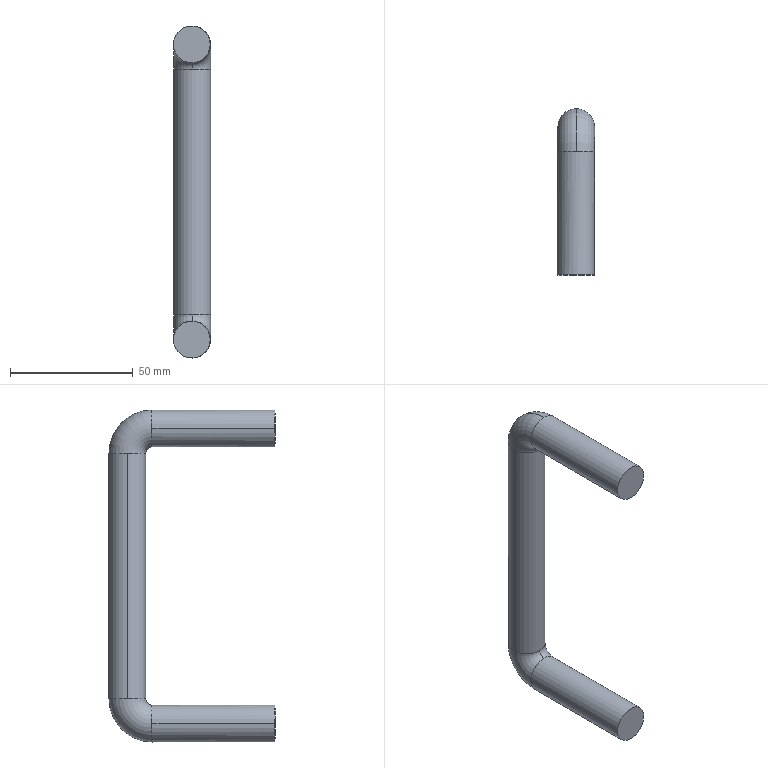Part | STEP file | Input 40 | 1 solid | 12 faces | box 15.178 x 67.522 x 135 mm | volume 40895 mm3 | cylinder 6 | torus 4 | plane 2 | commonest cylinder face diameters 15 x6
STEP:
#1=CARTESIAN_POINT('',(0.,0.,0.));
#2=DIRECTION('',(0.,0.,1.));
#3=DIRECTION('',(1.,0.,0.));
#4=AXIS2_PLACEMENT_3D('',#1,#2,#3);
#5=CARTESIAN_POINT('',(-3100.672,432.98,84.625));
#6=VERTEX_POINT('',#5);
#7=CARTESIAN_POINT('',(-3093.172,432.958,92.125));
#8=VERTEX_POINT('',#7);
#9=CARTESIAN_POINT('',(-3093.172,432.958,84.625));
#10=DIRECTION('',(0.002971,1.,0.));
#11=DIRECTION('',(-1.,0.002971,0.));
#12=AXIS2_PLACEMENT_3D('',#9,#10,#11);
#13=CIRCLE('',#12,7.5);
#14=CARTESIAN_POINT('',(-3093.172,432.958,74.625));
#15=DIRECTION('',(-1.,0.002971,0.));
#16=DIRECTION('',(0.,0.,1.));
#17=AXIS2_PLACEMENT_3D('',#14,#15,#16);
#18=TOROIDAL_SURFACE('',#17,10.,7.5);
#19=CARTESIAN_POINT('',(0.,1.571));
#20=CARTESIAN_POINT('',(0.,1.547));
#21=CARTESIAN_POINT('',(0.,1.499));
#22=CARTESIAN_POINT('',(0.,1.428));
#23=CARTESIAN_POINT('',(0.,1.357));
#24=CARTESIAN_POINT('',(0.,1.285));
#25=CARTESIAN_POINT('',(0.,1.214));
#26=CARTESIAN_POINT('',(0.,1.142));
#27=CARTESIAN_POINT('',(0.,1.071));
#28=CARTESIAN_POINT('',(0.,0.9996));
#29=CARTESIAN_POINT('',(0.,0.9282));
#30=CARTESIAN_POINT('',(0.,0.8568));
#31=CARTESIAN_POINT('',(0.,0.7854));
#32=CARTESIAN_POINT('',(0.,0.714));
#33=CARTESIAN_POINT('',(0.,0.6426));
#34=CARTESIAN_POINT('',(0.,0.5712));
#35=CARTESIAN_POINT('',(0.,0.4998));
#36=CARTESIAN_POINT('',(0.,0.4284));
#37=CARTESIAN_POINT('',(0.,0.357));
#38=CARTESIAN_POINT('',(0.,0.2856));
#39=CARTESIAN_POINT('',(0.,0.2142));
#40=CARTESIAN_POINT('',(0.,0.1428));
#41=CARTESIAN_POINT('',(0.,0.0714));
#42=CARTESIAN_POINT('',(0.,0.0238));
#43=CARTESIAN_POINT('',(0.,0.));
#44=B_SPLINE_CURVE_WITH_KNOTS('',3,(#19,#20,#21,#22,#23,#24,#25,#26,#27,#28,#29,#30,#31,#32,#33,#34,#35,#36,#37,#38,#39,#40,#41,#42,#43),.UNSPECIFIED.,.F.,.F.,(4,1,1,1,1,1,1,1,1,1,1,1,1,1,1,1,1,1,1,1,1,1,4),(0.,0.0714,0.1428,0.2142,0.2856,0.357,0.4284,0.4998,0.5712,0.6426,0.714,0.7854,0.8568,0.9282,0.9996,1.071,1.142,1.214,1.285,1.357,1.428,1.499,1.571),.QUASI_UNIFORM_KNOTS.);
#45=(GEOMETRIC_REPRESENTATION_CONTEXT(2)PARAMETRIC_REPRESENTATION_CONTEXT()REPRESENTATION_CONTEXT('',''));
#46=DEFINITIONAL_REPRESENTATION('',(#44),#45);
#47=PCURVE('',#18,#46);
#48=CARTESIAN_POINT('',(-3093.172,432.958,84.625));
#49=DIRECTION('',(-0.002971,-1.,0.));
#50=DIRECTION('',(1.,-0.002971,0.));
#51=AXIS2_PLACEMENT_3D('',#48,#49,#50);
#52=CYLINDRICAL_SURFACE('',#51,7.5);
#53=CARTESIAN_POINT('',(3.142,0.));
#54=DIRECTION('',(-1.,0.));
#55=VECTOR('',#54,1.);
#56=LINE('',#53,#55);
#57=(GEOMETRIC_REPRESENTATION_CONTEXT(2)PARAMETRIC_REPRESENTATION_CONTEXT()REPRESENTATION_CONTEXT('',''));
#58=DEFINITIONAL_REPRESENTATION('',(#56),#57);
#59=PCURVE('',#52,#58);
#60=SURFACE_CURVE('',#13,(#47,#59),.PCURVE_S1.);
#61=EDGE_CURVE('',#6,#8,#60,.T.);
#62=ORIENTED_EDGE('',*,*,#61,.T.);
#63=CARTESIAN_POINT('',(-3093.12,450.458,74.625));
#64=VERTEX_POINT('',#63);
#65=CARTESIAN_POINT('',(-3093.172,432.958,74.625));
#66=DIRECTION('',(-1.,0.002971,0.));
#67=DIRECTION('',(-0.002971,-1.,0.));
#68=AXIS2_PLACEMENT_3D('',#65,#66,#67);
#69=CIRCLE('',#68,17.5);
#70=CARTESIAN_POINT('',(-1.571,0.));
#71=DIRECTION('',(1.,0.));
#72=VECTOR('',#71,1.);
#73=LINE('',#70,#72);
#74=(GEOMETRIC_REPRESENTATION_CONTEXT(2)PARAMETRIC_REPRESENTATION_CONTEXT()REPRESENTATION_CONTEXT('',''));
#75=DEFINITIONAL_REPRESENTATION('',(#73),#74);
#76=PCURVE('',#18,#75);
#77=CARTESIAN_POINT('',(-3093.172,432.958,74.625));
#78=DIRECTION('',(-1.,0.002971,0.));
#79=DIRECTION('',(0.,0.,1.));
#80=AXIS2_PLACEMENT_3D('',#77,#78,#79);
#81=TOROIDAL_SURFACE('',#80,10.,7.5);
#82=CARTESIAN_POINT('',(-1.571,6.283));
#83=DIRECTION('',(1.,0.));
#84=VECTOR('',#83,1.);
#85=LINE('',#82,#84);
#86=(GEOMETRIC_REPRESENTATION_CONTEXT(2)PARAMETRIC_REPRESENTATION_CONTEXT()REPRESENTATION_CONTEXT('',''));
#87=DEFINITIONAL_REPRESENTATION('',(#85),#86);
#88=PCURVE('',#81,#87);
#89=SURFACE_CURVE('',#69,(#76,#88),.PCURVE_S1.);
#90=EDGE_CURVE('',#8,#64,#89,.T.);
#91=ORIENTED_EDGE('',*,*,#90,.T.);
#92=CARTESIAN_POINT('',(-3100.643,442.98,74.625));
#93=VERTEX_POINT('',#92);
#94=CARTESIAN_POINT('',(-3093.143,442.958,74.625));
#95=DIRECTION('',(0.,0.,-1.));
#96=DIRECTION('',(-1.,0.002971,0.));
#97=AXIS2_PLACEMENT_3D('',#94,#95,#96);
#98=CIRCLE('',#97,7.5);
#99=CARTESIAN_POINT('',(1.571,1.571));
#100=DIRECTION('',(0.,-1.));
#101=VECTOR('',#100,1.);
#102=LINE('',#99,#101);
#103=(GEOMETRIC_REPRESENTATION_CONTEXT(2)PARAMETRIC_REPRESENTATION_CONTEXT()REPRESENTATION_CONTEXT('',''));
#104=DEFINITIONAL_REPRESENTATION('',(#102),#103);
#105=PCURVE('',#18,#104);
#106=CARTESIAN_POINT('',(-3093.143,442.958,74.625));
#107=DIRECTION('',(0.,0.,-1.));
#108=DIRECTION('',(-1.,0.002971,0.));
#109=AXIS2_PLACEMENT_3D('',#106,#107,#108);
#110=CYLINDRICAL_SURFACE('',#109,7.5);
#111=CARTESIAN_POINT('',(0.,0.));
#112=DIRECTION('',(1.,0.));
#113=VECTOR('',#112,1.);
#114=LINE('',#111,#113);
#115=(GEOMETRIC_REPRESENTATION_CONTEXT(2)PARAMETRIC_REPRESENTATION_CONTEXT()REPRESENTATION_CONTEXT('',''));
#116=DEFINITIONAL_REPRESENTATION('',(#114),#115);
#117=PCURVE('',#110,#116);
#118=SURFACE_CURVE('',#98,(#105,#117),.PCURVE_S1.);
#119=EDGE_CURVE('',#93,#64,#118,.T.);
#120=ORIENTED_EDGE('',*,*,#119,.F.);
#121=CARTESIAN_POINT('',(-3093.165,435.458,74.625));
#122=VERTEX_POINT('',#121);
#123=CARTESIAN_POINT('',(-3093.143,442.958,74.625));
#124=DIRECTION('',(0.,0.,-1.));
#125=DIRECTION('',(-1.,0.002971,0.));
#126=AXIS2_PLACEMENT_3D('',#123,#124,#125);
#127=CIRCLE('',#126,7.5);
#128=CARTESIAN_POINT('',(1.571,7.854));
#129=DIRECTION('',(0.,-1.));
#130=VECTOR('',#129,1.);
#131=LINE('',#128,#130);
#132=(GEOMETRIC_REPRESENTATION_CONTEXT(2)PARAMETRIC_REPRESENTATION_CONTEXT()REPRESENTATION_CONTEXT('',''));
#133=DEFINITIONAL_REPRESENTATION('',(#131),#132);
#134=PCURVE('',#18,#133);
#135=CARTESIAN_POINT('',(-3093.143,442.958,74.625));
#136=DIRECTION('',(0.,0.,-1.));
#137=DIRECTION('',(-1.,0.002971,0.));
#138=AXIS2_PLACEMENT_3D('',#135,#136,#137);
#139=CYLINDRICAL_SURFACE('',#138,7.5);
#140=CARTESIAN_POINT('',(0.,0.));
#141=DIRECTION('',(1.,0.));
#142=VECTOR('',#141,1.);
#143=LINE('',#140,#142);
#144=(GEOMETRIC_REPRESENTATION_CONTEXT(2)PARAMETRIC_REPRESENTATION_CONTEXT()REPRESENTATION_CONTEXT('',''));
#145=DEFINITIONAL_REPRESENTATION('',(#143),#144);
#146=PCURVE('',#139,#145);
#147=SURFACE_CURVE('',#127,(#134,#146),.PCURVE_S1.);
#148=EDGE_CURVE('',#122,#93,#147,.T.);
#149=ORIENTED_EDGE('',*,*,#148,.F.);
#150=CARTESIAN_POINT('',(-3093.172,432.958,77.125));
#151=VERTEX_POINT('',#150);
#152=CARTESIAN_POINT('',(-3093.172,432.958,74.625));
#153=DIRECTION('',(-1.,0.002971,0.));
#154=DIRECTION('',(-0.002971,-1.,0.));
#155=AXIS2_PLACEMENT_3D('',#152,#153,#154);
#156=CIRCLE('',#155,2.5);
#157=CARTESIAN_POINT('',(-1.571,3.142));
#158=DIRECTION('',(1.,0.));
#159=VECTOR('',#158,1.);
#160=LINE('',#157,#159);
#161=(GEOMETRIC_REPRESENTATION_CONTEXT(2)PARAMETRIC_REPRESENTATION_CONTEXT()REPRESENTATION_CONTEXT('',''));
#162=DEFINITIONAL_REPRESENTATION('',(#160),#161);
#163=PCURVE('',#18,#162);
#164=CARTESIAN_POINT('',(-1.571,3.142));
#165=DIRECTION('',(1.,0.));
#166=VECTOR('',#165,1.);
#167=LINE('',#164,#166);
#168=(GEOMETRIC_REPRESENTATION_CONTEXT(2)PARAMETRIC_REPRESENTATION_CONTEXT()REPRESENTATION_CONTEXT('',''));
#169=DEFINITIONAL_REPRESENTATION('',(#167),#168);
#170=PCURVE('',#81,#169);
#171=SURFACE_CURVE('',#156,(#163,#170),.PCURVE_S1.);
#172=EDGE_CURVE('',#151,#122,#171,.T.);
#173=ORIENTED_EDGE('',*,*,#172,.F.);
#174=CARTESIAN_POINT('',(-3093.172,432.958,84.625));
#175=DIRECTION('',(0.002971,1.,0.));
#176=DIRECTION('',(-1.,0.002971,0.));
#177=AXIS2_PLACEMENT_3D('',#174,#175,#176);
#178=CIRCLE('',#177,7.5);
#179=CARTESIAN_POINT('',(0.,7.854));
#180=DIRECTION('',(0.,-1.));
#181=VECTOR('',#180,1.);
#182=LINE('',#179,#181);
#183=(GEOMETRIC_REPRESENTATION_CONTEXT(2)PARAMETRIC_REPRESENTATION_CONTEXT()REPRESENTATION_CONTEXT('',''));
#184=DEFINITIONAL_REPRESENTATION('',(#182),#183);
#185=PCURVE('',#18,#184);
#186=CARTESIAN_POINT('',(-3093.172,432.958,84.625));
#187=DIRECTION('',(-0.002971,-1.,0.));
#188=DIRECTION('',(1.,-0.002971,0.));
#189=AXIS2_PLACEMENT_3D('',#186,#187,#188);
#190=CYLINDRICAL_SURFACE('',#189,7.5);
#191=CARTESIAN_POINT('',(9.425,0.));
#192=DIRECTION('',(-1.,0.));
#193=VECTOR('',#192,1.);
#194=LINE('',#191,#193);
#195=(GEOMETRIC_REPRESENTATION_CONTEXT(2)PARAMETRIC_REPRESENTATION_CONTEXT()REPRESENTATION_CONTEXT('',''));
#196=DEFINITIONAL_REPRESENTATION('',(#194),#195);
#197=PCURVE('',#190,#196);
#198=SURFACE_CURVE('',#178,(#185,#197),.PCURVE_S1.);
#199=EDGE_CURVE('',#151,#6,#198,.T.);
#200=ORIENTED_EDGE('',*,*,#199,.T.);
#201=EDGE_LOOP('',(#62,#91,#120,#149,#173,#200));
#202=FACE_BOUND('',#201,.T.);
#203=ADVANCED_FACE('',(#202),#18,.T.);
#204=CARTESIAN_POINT('',(-3100.643,442.98,-25.375));
#205=VERTEX_POINT('',#204);
#206=CARTESIAN_POINT('',(-3093.12,450.458,-25.375));
#207=VERTEX_POINT('',#206);
#208=CARTESIAN_POINT('',(-3093.143,442.958,-25.375));
#209=DIRECTION('',(0.,0.,-1.));
#210=DIRECTION('',(-1.,0.002971,0.));
#211=AXIS2_PLACEMENT_3D('',#208,#209,#210);
#212=CIRCLE('',#211,7.5);
#213=CARTESIAN_POINT('',(-3093.172,432.958,-25.375));
#214=DIRECTION('',(-1.,0.002971,0.));
#215=DIRECTION('',(0.,0.,1.));
#216=AXIS2_PLACEMENT_3D('',#213,#214,#215);
#217=TOROIDAL_SURFACE('',#216,10.,7.5);
#218=CARTESIAN_POINT('',(1.571,1.571));
#219=DIRECTION('',(0.,-1.));
#220=VECTOR('',#219,1.);
#221=LINE('',#218,#220);
#222=(GEOMETRIC_REPRESENTATION_CONTEXT(2)PARAMETRIC_REPRESENTATION_CONTEXT()REPRESENTATION_CONTEXT('',''));
#223=DEFINITIONAL_REPRESENTATION('',(#221),#222);
#224=PCURVE('',#217,#223);
#225=CARTESIAN_POINT('',(0.,100.));
#226=DIRECTION('',(1.,0.));
#227=VECTOR('',#226,1.);
#228=LINE('',#225,#227);
#229=(GEOMETRIC_REPRESENTATION_CONTEXT(2)PARAMETRIC_REPRESENTATION_CONTEXT()REPRESENTATION_CONTEXT('',''));
#230=DEFINITIONAL_REPRESENTATION('',(#228),#229);
#231=PCURVE('',#110,#230);
#232=SURFACE_CURVE('',#212,(#224,#231),.PCURVE_S1.);
#233=EDGE_CURVE('',#205,#207,#232,.T.);
#234=ORIENTED_EDGE('',*,*,#233,.T.);
#235=CARTESIAN_POINT('',(-3093.172,432.958,-42.875));
#236=VERTEX_POINT('',#235);
#237=CARTESIAN_POINT('',(-3093.172,432.958,-25.375));
#238=DIRECTION('',(-1.,0.002971,0.));
#239=DIRECTION('',(-0.002971,-1.,0.));
#240=AXIS2_PLACEMENT_3D('',#237,#238,#239);
#241=CIRCLE('',#240,17.5);
#242=CARTESIAN_POINT('',(-1.571,0.));
#243=DIRECTION('',(1.,0.));
#244=VECTOR('',#243,1.);
#245=LINE('',#242,#244);
#246=(GEOMETRIC_REPRESENTATION_CONTEXT(2)PARAMETRIC_REPRESENTATION_CONTEXT()REPRESENTATION_CONTEXT('',''));
#247=DEFINITIONAL_REPRESENTATION('',(#245),#246);
#248=PCURVE('',#217,#247);
#249=CARTESIAN_POINT('',(-3093.172,432.958,-25.375));
#250=DIRECTION('',(-1.,0.002971,0.));
#251=DIRECTION('',(0.,0.,1.));
#252=AXIS2_PLACEMENT_3D('',#249,#250,#251);
#253=TOROIDAL_SURFACE('',#252,10.,7.5);
#254=CARTESIAN_POINT('',(-1.571,6.283));
#255=DIRECTION('',(1.,0.));
#256=VECTOR('',#255,1.);
#257=LINE('',#254,#256);
#258=(GEOMETRIC_REPRESENTATION_CONTEXT(2)PARAMETRIC_REPRESENTATION_CONTEXT()REPRESENTATION_CONTEXT('',''));
#259=DEFINITIONAL_REPRESENTATION('',(#257),#258);
#260=PCURVE('',#253,#259);
#261=SURFACE_CURVE('',#241,(#248,#260),.PCURVE_S1.);
#262=EDGE_CURVE('',#207,#236,#261,.T.);
#263=ORIENTED_EDGE('',*,*,#262,.T.);
#264=CARTESIAN_POINT('',(-3100.672,432.98,-35.375));
#265=VERTEX_POINT('',#264);
#266=CARTESIAN_POINT('',(-3093.172,432.958,-35.375));
#267=DIRECTION('',(-0.002971,-1.,0.));
#268=DIRECTION('',(-1.,0.002971,0.));
#269=AXIS2_PLACEMENT_3D('',#266,#267,#268);
#270=CIRCLE('',#269,7.5);
#271=CARTESIAN_POINT('',(3.142,1.571));
#272=DIRECTION('',(0.,-1.));
#273=VECTOR('',#272,1.);
#274=LINE('',#271,#273);
#275=(GEOMETRIC_REPRESENTATION_CONTEXT(2)PARAMETRIC_REPRESENTATION_CONTEXT()REPRESENTATION_CONTEXT('',''));
#276=DEFINITIONAL_REPRESENTATION('',(#274),#275);
#277=PCURVE('',#217,#276);
#278=CARTESIAN_POINT('',(-3093.172,432.958,-35.375));
#279=DIRECTION('',(-0.002971,-1.,0.));
#280=DIRECTION('',(1.,-0.002971,0.));
#281=AXIS2_PLACEMENT_3D('',#278,#279,#280);
#282=CYLINDRICAL_SURFACE('',#281,7.5);
#283=CARTESIAN_POINT('',(3.142,0.));
#284=DIRECTION('',(1.,0.));
#285=VECTOR('',#284,1.);
#286=LINE('',#283,#285);
#287=(GEOMETRIC_REPRESENTATION_CONTEXT(2)PARAMETRIC_REPRESENTATION_CONTEXT()REPRESENTATION_CONTEXT('',''));
#288=DEFINITIONAL_REPRESENTATION('',(#286),#287);
#289=PCURVE('',#282,#288);
#290=SURFACE_CURVE('',#270,(#277,#289),.PCURVE_S1.);
#291=EDGE_CURVE('',#265,#236,#290,.T.);
#292=ORIENTED_EDGE('',*,*,#291,.F.);
#293=CARTESIAN_POINT('',(-3093.172,432.958,-27.875));
#294=VERTEX_POINT('',#293);
#295=CARTESIAN_POINT('',(-3093.172,432.958,-35.375));
#296=DIRECTION('',(-0.002971,-1.,0.));
#297=DIRECTION('',(-1.,0.002971,0.));
#298=AXIS2_PLACEMENT_3D('',#295,#296,#297);
#299=CIRCLE('',#298,7.5);
#300=CARTESIAN_POINT('',(3.142,7.854));
#301=DIRECTION('',(0.,-1.));
#302=VECTOR('',#301,1.);
#303=LINE('',#300,#302);
#304=(GEOMETRIC_REPRESENTATION_CONTEXT(2)PARAMETRIC_REPRESENTATION_CONTEXT()REPRESENTATION_CONTEXT('',''));
#305=DEFINITIONAL_REPRESENTATION('',(#303),#304);
#306=PCURVE('',#217,#305);
#307=CARTESIAN_POINT('',(-3093.172,432.958,-35.375));
#308=DIRECTION('',(-0.002971,-1.,0.));
#309=DIRECTION('',(1.,-0.002971,0.));
#310=AXIS2_PLACEMENT_3D('',#307,#308,#309);
#311=CYLINDRICAL_SURFACE('',#310,7.5);
#312=CARTESIAN_POINT('',(-3.142,0.));
#313=DIRECTION('',(1.,0.));
#314=VECTOR('',#313,1.);
#315=LINE('',#312,#314);
#316=(GEOMETRIC_REPRESENTATION_CONTEXT(2)PARAMETRIC_REPRESENTATION_CONTEXT()REPRESENTATION_CONTEXT('',''));
#317=DEFINITIONAL_REPRESENTATION('',(#315),#316);
#318=PCURVE('',#311,#317);
#319=SURFACE_CURVE('',#299,(#306,#318),.PCURVE_S1.);
#320=EDGE_CURVE('',#294,#265,#319,.T.);
#321=ORIENTED_EDGE('',*,*,#320,.F.);
#322=CARTESIAN_POINT('',(-3093.165,435.458,-25.375));
#323=VERTEX_POINT('',#322);
#324=CARTESIAN_POINT('',(-3093.172,432.958,-25.375));
#325=DIRECTION('',(-1.,0.002971,0.));
#326=DIRECTION('',(-0.002971,-1.,0.));
#327=AXIS2_PLACEMENT_3D('',#324,#325,#326);
#328=CIRCLE('',#327,2.5);
#329=CARTESIAN_POINT('',(-1.571,3.142));
#330=DIRECTION('',(1.,0.));
#331=VECTOR('',#330,1.);
#332=LINE('',#329,#331);
#333=(GEOMETRIC_REPRESENTATION_CONTEXT(2)PARAMETRIC_REPRESENTATION_CONTEXT()REPRESENTATION_CONTEXT('',''));
#334=DEFINITIONAL_REPRESENTATION('',(#332),#333);
#335=PCURVE('',#217,#334);
#336=CARTESIAN_POINT('',(-1.571,3.142));
#337=DIRECTION('',(1.,0.));
#338=VECTOR('',#337,1.);
#339=LINE('',#336,#338);
#340=(GEOMETRIC_REPRESENTATION_CONTEXT(2)PARAMETRIC_REPRESENTATION_CONTEXT()REPRESENTATION_CONTEXT('',''));
#341=DEFINITIONAL_REPRESENTATION('',(#339),#340);
#342=PCURVE('',#253,#341);
#343=SURFACE_CURVE('',#328,(#335,#342),.PCURVE_S1.);
#344=EDGE_CURVE('',#323,#294,#343,.T.);
#345=ORIENTED_EDGE('',*,*,#344,.F.);
#346=CARTESIAN_POINT('',(-3093.143,442.958,-25.375));
#347=DIRECTION('',(0.,0.,-1.));
#348=DIRECTION('',(-1.,0.002971,0.));
#349=AXIS2_PLACEMENT_3D('',#346,#347,#348);
#350=CIRCLE('',#349,7.5);
#351=CARTESIAN_POINT('',(1.571,7.854));
#352=DIRECTION('',(0.,-1.));
#353=VECTOR('',#352,1.);
#354=LINE('',#351,#353);
#355=(GEOMETRIC_REPRESENTATION_CONTEXT(2)PARAMETRIC_REPRESENTATION_CONTEXT()REPRESENTATION_CONTEXT('',''));
#356=DEFINITIONAL_REPRESENTATION('',(#354),#355);
#357=PCURVE('',#217,#356);
#358=CARTESIAN_POINT('',(0.,100.));
#359=DIRECTION('',(1.,0.));
#360=VECTOR('',#359,1.);
#361=LINE('',#358,#360);
#362=(GEOMETRIC_REPRESENTATION_CONTEXT(2)PARAMETRIC_REPRESENTATION_CONTEXT()REPRESENTATION_CONTEXT('',''));
#363=DEFINITIONAL_REPRESENTATION('',(#361),#362);
#364=PCURVE('',#139,#363);
#365=SURFACE_CURVE('',#350,(#357,#364),.PCURVE_S1.);
#366=EDGE_CURVE('',#323,#205,#365,.T.);
#367=ORIENTED_EDGE('',*,*,#366,.T.);
#368=EDGE_LOOP('',(#234,#263,#292,#321,#345,#367));
#369=FACE_BOUND('',#368,.T.);
#370=ADVANCED_FACE('',(#369),#217,.T.);
#371=ORIENTED_EDGE('',*,*,#61,.F.);
#372=CARTESIAN_POINT('',(-3100.821,382.98,84.625));
#373=VERTEX_POINT('',#372);
#374=CARTESIAN_POINT('',(-3100.672,432.98,84.625));
#375=DIRECTION('',(-0.002971,-1.,0.));
#376=VECTOR('',#375,1.);
#377=LINE('',#374,#376);
#378=CARTESIAN_POINT('',(3.142,0.));
#379=DIRECTION('',(0.,1.));
#380=VECTOR('',#379,1.);
#381=LINE('',#378,#380);
#382=(GEOMETRIC_REPRESENTATION_CONTEXT(2)PARAMETRIC_REPRESENTATION_CONTEXT()REPRESENTATION_CONTEXT('',''));
#383=DEFINITIONAL_REPRESENTATION('',(#381),#382);
#384=PCURVE('',#52,#383);
#385=CARTESIAN_POINT('',(3.142,0.));
#386=DIRECTION('',(0.,1.));
#387=VECTOR('',#386,1.);
#388=LINE('',#385,#387);
#389=(GEOMETRIC_REPRESENTATION_CONTEXT(2)PARAMETRIC_REPRESENTATION_CONTEXT()REPRESENTATION_CONTEXT('',''));
#390=DEFINITIONAL_REPRESENTATION('',(#388),#389);
#391=PCURVE('',#190,#390);
#392=SURFACE_CURVE('',#377,(#384,#391),.PCURVE_S1.);
#393=EDGE_CURVE('',#6,#373,#392,.T.);
#394=ORIENTED_EDGE('',*,*,#393,.T.);
#395=CARTESIAN_POINT('',(-3085.821,382.936,84.625));
#396=VERTEX_POINT('',#395);
#397=CARTESIAN_POINT('',(-3093.321,382.958,84.625));
#398=DIRECTION('',(0.002971,1.,0.));
#399=DIRECTION('',(-1.,0.002971,0.));
#400=AXIS2_PLACEMENT_3D('',#397,#398,#399);
#401=CIRCLE('',#400,7.5);
#402=CARTESIAN_POINT('',(3.142,50.));
#403=DIRECTION('',(-1.,0.));
#404=VECTOR('',#403,1.);
#405=LINE('',#402,#404);
#406=(GEOMETRIC_REPRESENTATION_CONTEXT(2)PARAMETRIC_REPRESENTATION_CONTEXT()REPRESENTATION_CONTEXT('',''));
#407=DEFINITIONAL_REPRESENTATION('',(#405),#406);
#408=PCURVE('',#52,#407);
#409=CARTESIAN_POINT('',(-3093.321,382.958,84.625));
#410=DIRECTION('',(0.002971,1.,0.));
#411=DIRECTION('',(-1.,0.002971,0.));
#412=AXIS2_PLACEMENT_3D('',#409,#410,#411);
#413=PLANE('',#412);
#414=CARTESIAN_POINT('',(0.,0.));
#415=DIRECTION('',(1.,0.));
#416=AXIS2_PLACEMENT_2D('',#414,#415);
#417=CIRCLE('',#416,7.5);
#418=(GEOMETRIC_REPRESENTATION_CONTEXT(2)PARAMETRIC_REPRESENTATION_CONTEXT()REPRESENTATION_CONTEXT('',''));
#419=DEFINITIONAL_REPRESENTATION('',(#417),#418);
#420=PCURVE('',#413,#419);
#421=SURFACE_CURVE('',#401,(#408,#420),.PCURVE_S1.);
#422=EDGE_CURVE('',#373,#396,#421,.T.);
#423=ORIENTED_EDGE('',*,*,#422,.T.);
#424=CARTESIAN_POINT('',(-3085.672,432.936,84.625));
#425=VERTEX_POINT('',#424);
#426=CARTESIAN_POINT('',(-3085.672,432.936,84.625));
#427=DIRECTION('',(-0.002971,-1.,0.));
#428=VECTOR('',#427,1.);
#429=LINE('',#426,#428);
#430=CARTESIAN_POINT('',(0.,0.));
#431=DIRECTION('',(0.,1.));
#432=VECTOR('',#431,1.);
#433=LINE('',#430,#432);
#434=(GEOMETRIC_REPRESENTATION_CONTEXT(2)PARAMETRIC_REPRESENTATION_CONTEXT()REPRESENTATION_CONTEXT('',''));
#435=DEFINITIONAL_REPRESENTATION('',(#433),#434);
#436=PCURVE('',#52,#435);
#437=CARTESIAN_POINT('',(6.283,0.));
#438=DIRECTION('',(0.,1.));
#439=VECTOR('',#438,1.);
#440=LINE('',#437,#439);
#441=(GEOMETRIC_REPRESENTATION_CONTEXT(2)PARAMETRIC_REPRESENTATION_CONTEXT()REPRESENTATION_CONTEXT('',''));
#442=DEFINITIONAL_REPRESENTATION('',(#440),#441);
#443=PCURVE('',#190,#442);
#444=SURFACE_CURVE('',#429,(#436,#443),.PCURVE_S1.);
#445=EDGE_CURVE('',#425,#396,#444,.T.);
#446=ORIENTED_EDGE('',*,*,#445,.F.);
#447=CARTESIAN_POINT('',(-3093.172,432.958,84.625));
#448=DIRECTION('',(0.002971,1.,0.));
#449=DIRECTION('',(-1.,0.002971,0.));
#450=AXIS2_PLACEMENT_3D('',#447,#448,#449);
#451=CIRCLE('',#450,7.5);
#452=CARTESIAN_POINT('',(3.142,0.));
#453=DIRECTION('',(-1.,0.));
#454=VECTOR('',#453,1.);
#455=LINE('',#452,#454);
#456=(GEOMETRIC_REPRESENTATION_CONTEXT(2)PARAMETRIC_REPRESENTATION_CONTEXT()REPRESENTATION_CONTEXT('',''));
#457=DEFINITIONAL_REPRESENTATION('',(#455),#456);
#458=PCURVE('',#52,#457);
#459=CARTESIAN_POINT('',(0.,7.854));
#460=DIRECTION('',(0.,-1.));
#461=VECTOR('',#460,1.);
#462=LINE('',#459,#461);
#463=(GEOMETRIC_REPRESENTATION_CONTEXT(2)PARAMETRIC_REPRESENTATION_CONTEXT()REPRESENTATION_CONTEXT('',''));
#464=DEFINITIONAL_REPRESENTATION('',(#462),#463);
#465=PCURVE('',#81,#464);
#466=SURFACE_CURVE('',#451,(#458,#465),.PCURVE_S1.);
#467=EDGE_CURVE('',#8,#425,#466,.T.);
#468=ORIENTED_EDGE('',*,*,#467,.F.);
#469=EDGE_LOOP('',(#371,#394,#423,#446,#468));
#470=FACE_BOUND('',#469,.T.);
#471=ADVANCED_FACE('',(#470),#52,.T.);
#472=ORIENTED_EDGE('',*,*,#119,.T.);
#473=CARTESIAN_POINT('',(-3085.643,442.935,74.625));
#474=VERTEX_POINT('',#473);
#475=CARTESIAN_POINT('',(-3093.143,442.958,74.625));
#476=DIRECTION('',(0.,0.,-1.));
#477=DIRECTION('',(-1.,0.002971,0.));
#478=AXIS2_PLACEMENT_3D('',#475,#476,#477);
#479=CIRCLE('',#478,7.5);
#480=CARTESIAN_POINT('',(0.,0.));
#481=DIRECTION('',(1.,0.));
#482=VECTOR('',#481,1.);
#483=LINE('',#480,#482);
#484=(GEOMETRIC_REPRESENTATION_CONTEXT(2)PARAMETRIC_REPRESENTATION_CONTEXT()REPRESENTATION_CONTEXT('',''));
#485=DEFINITIONAL_REPRESENTATION('',(#483),#484);
#486=PCURVE('',#110,#485);
#487=CARTESIAN_POINT('',(1.571,7.854));
#488=DIRECTION('',(0.,-1.));
#489=VECTOR('',#488,1.);
#490=LINE('',#487,#489);
#491=(GEOMETRIC_REPRESENTATION_CONTEXT(2)PARAMETRIC_REPRESENTATION_CONTEXT()REPRESENTATION_CONTEXT('',''));
#492=DEFINITIONAL_REPRESENTATION('',(#490),#491);
#493=PCURVE('',#81,#492);
#494=SURFACE_CURVE('',#479,(#486,#493),.PCURVE_S1.);
#495=EDGE_CURVE('',#64,#474,#494,.T.);
#496=ORIENTED_EDGE('',*,*,#495,.T.);
#497=CARTESIAN_POINT('',(-3085.643,442.935,-25.375));
#498=VERTEX_POINT('',#497);
#499=CARTESIAN_POINT('',(-3085.643,442.935,74.625));
#500=DIRECTION('',(0.,0.,-1.));
#501=VECTOR('',#500,1.);
#502=LINE('',#499,#501);
#503=CARTESIAN_POINT('',(3.142,0.));
#504=DIRECTION('',(0.,1.));
#505=VECTOR('',#504,1.);
#506=LINE('',#503,#505);
#507=(GEOMETRIC_REPRESENTATION_CONTEXT(2)PARAMETRIC_REPRESENTATION_CONTEXT()REPRESENTATION_CONTEXT('',''));
#508=DEFINITIONAL_REPRESENTATION('',(#506),#507);
#509=PCURVE('',#110,#508);
#510=CARTESIAN_POINT('',(3.142,0.));
#511=DIRECTION('',(0.,1.));
#512=VECTOR('',#511,1.);
#513=LINE('',#510,#512);
#514=(GEOMETRIC_REPRESENTATION_CONTEXT(2)PARAMETRIC_REPRESENTATION_CONTEXT()REPRESENTATION_CONTEXT('',''));
#515=DEFINITIONAL_REPRESENTATION('',(#513),#514);
#516=PCURVE('',#139,#515);
#517=SURFACE_CURVE('',#502,(#509,#516),.PCURVE_S1.);
#518=EDGE_CURVE('',#474,#498,#517,.T.);
#519=ORIENTED_EDGE('',*,*,#518,.T.);
#520=CARTESIAN_POINT('',(-3093.143,442.958,-25.375));
#521=DIRECTION('',(0.,0.,-1.));
#522=DIRECTION('',(-1.,0.002971,0.));
#523=AXIS2_PLACEMENT_3D('',#520,#521,#522);
#524=CIRCLE('',#523,7.5);
#525=CARTESIAN_POINT('',(0.,100.));
#526=DIRECTION('',(1.,0.));
#527=VECTOR('',#526,1.);
#528=LINE('',#525,#527);
#529=(GEOMETRIC_REPRESENTATION_CONTEXT(2)PARAMETRIC_REPRESENTATION_CONTEXT()REPRESENTATION_CONTEXT('',''));
#530=DEFINITIONAL_REPRESENTATION('',(#528),#529);
#531=PCURVE('',#110,#530);
#532=CARTESIAN_POINT('',(1.571,7.854));
#533=DIRECTION('',(0.,-1.));
#534=VECTOR('',#533,1.);
#535=LINE('',#532,#534);
#536=(GEOMETRIC_REPRESENTATION_CONTEXT(2)PARAMETRIC_REPRESENTATION_CONTEXT()REPRESENTATION_CONTEXT('',''));
#537=DEFINITIONAL_REPRESENTATION('',(#535),#536);
#538=PCURVE('',#253,#537);
#539=SURFACE_CURVE('',#524,(#531,#538),.PCURVE_S1.);
#540=EDGE_CURVE('',#207,#498,#539,.T.);
#541=ORIENTED_EDGE('',*,*,#540,.F.);
#542=ORIENTED_EDGE('',*,*,#233,.F.);
#543=CARTESIAN_POINT('',(-3100.643,442.98,74.625));
#544=DIRECTION('',(0.,0.,-1.));
#545=VECTOR('',#544,1.);
#546=LINE('',#543,#545);
#547=CARTESIAN_POINT('',(0.,0.));
#548=DIRECTION('',(0.,1.));
#549=VECTOR('',#548,1.);
#550=LINE('',#547,#549);
#551=(GEOMETRIC_REPRESENTATION_CONTEXT(2)PARAMETRIC_REPRESENTATION_CONTEXT()REPRESENTATION_CONTEXT('',''));
#552=DEFINITIONAL_REPRESENTATION('',(#550),#551);
#553=PCURVE('',#110,#552);
#554=CARTESIAN_POINT('',(6.283,0.));
#555=DIRECTION('',(0.,1.));
#556=VECTOR('',#555,1.);
#557=LINE('',#554,#556);
#558=(GEOMETRIC_REPRESENTATION_CONTEXT(2)PARAMETRIC_REPRESENTATION_CONTEXT()REPRESENTATION_CONTEXT('',''));
#559=DEFINITIONAL_REPRESENTATION('',(#557),#558);
#560=PCURVE('',#139,#559);
#561=SURFACE_CURVE('',#546,(#553,#560),.PCURVE_S1.);
#562=EDGE_CURVE('',#93,#205,#561,.T.);
#563=ORIENTED_EDGE('',*,*,#562,.F.);
#564=EDGE_LOOP('',(#472,#496,#519,#541,#542,#563));
#565=FACE_BOUND('',#564,.T.);
#566=ADVANCED_FACE('',(#565),#110,.T.);
#567=CARTESIAN_POINT('',(-3085.672,432.936,-35.375));
#568=VERTEX_POINT('',#567);
#569=CARTESIAN_POINT('',(-3093.172,432.958,-35.375));
#570=DIRECTION('',(-0.002971,-1.,0.));
#571=DIRECTION('',(-1.,0.002971,0.));
#572=AXIS2_PLACEMENT_3D('',#569,#570,#571);
#573=CIRCLE('',#572,7.5);
#574=CARTESIAN_POINT('',(-3.142,0.));
#575=DIRECTION('',(1.,0.));
#576=VECTOR('',#575,1.);
#577=LINE('',#574,#576);
#578=(GEOMETRIC_REPRESENTATION_CONTEXT(2)PARAMETRIC_REPRESENTATION_CONTEXT()REPRESENTATION_CONTEXT('',''));
#579=DEFINITIONAL_REPRESENTATION('',(#577),#578);
#580=PCURVE('',#311,#579);
#581=CARTESIAN_POINT('',(3.142,7.854));
#582=DIRECTION('',(0.,-1.));
#583=VECTOR('',#582,1.);
#584=LINE('',#581,#583);
#585=(GEOMETRIC_REPRESENTATION_CONTEXT(2)PARAMETRIC_REPRESENTATION_CONTEXT()REPRESENTATION_CONTEXT('',''));
#586=DEFINITIONAL_REPRESENTATION('',(#584),#585);
#587=PCURVE('',#253,#586);
#588=SURFACE_CURVE('',#573,(#580,#587),.PCURVE_S1.);
#589=EDGE_CURVE('',#568,#294,#588,.T.);
#590=ORIENTED_EDGE('',*,*,#589,.T.);
#591=ORIENTED_EDGE('',*,*,#320,.T.);
#592=CARTESIAN_POINT('',(-3100.821,382.98,-35.375));
#593=VERTEX_POINT('',#592);
#594=CARTESIAN_POINT('',(-3100.672,432.98,-35.375));
#595=DIRECTION('',(-0.002971,-1.,0.));
#596=VECTOR('',#595,1.);
#597=LINE('',#594,#596);
#598=CARTESIAN_POINT('',(3.142,0.));
#599=DIRECTION('',(0.,1.));
#600=VECTOR('',#599,1.);
#601=LINE('',#598,#600);
#602=(GEOMETRIC_REPRESENTATION_CONTEXT(2)PARAMETRIC_REPRESENTATION_CONTEXT()REPRESENTATION_CONTEXT('',''));
#603=DEFINITIONAL_REPRESENTATION('',(#601),#602);
#604=PCURVE('',#311,#603);
#605=CARTESIAN_POINT('',(3.142,0.));
#606=DIRECTION('',(0.,1.));
#607=VECTOR('',#606,1.);
#608=LINE('',#605,#607);
#609=(GEOMETRIC_REPRESENTATION_CONTEXT(2)PARAMETRIC_REPRESENTATION_CONTEXT()REPRESENTATION_CONTEXT('',''));
#610=DEFINITIONAL_REPRESENTATION('',(#608),#609);
#611=PCURVE('',#282,#610);
#612=SURFACE_CURVE('',#597,(#604,#611),.PCURVE_S1.);
#613=EDGE_CURVE('',#265,#593,#612,.T.);
#614=ORIENTED_EDGE('',*,*,#613,.T.);
#615=CARTESIAN_POINT('',(-3085.821,382.936,-35.375));
#616=VERTEX_POINT('',#615);
#617=CARTESIAN_POINT('',(-3093.321,382.958,-35.375));
#618=DIRECTION('',(-0.002971,-1.,0.));
#619=DIRECTION('',(-1.,0.002971,0.));
#620=AXIS2_PLACEMENT_3D('',#617,#618,#619);
#621=CIRCLE('',#620,7.5);
#622=CARTESIAN_POINT('',(-3.142,50.));
#623=DIRECTION('',(1.,0.));
#624=VECTOR('',#623,1.);
#625=LINE('',#622,#624);
#626=(GEOMETRIC_REPRESENTATION_CONTEXT(2)PARAMETRIC_REPRESENTATION_CONTEXT()REPRESENTATION_CONTEXT('',''));
#627=DEFINITIONAL_REPRESENTATION('',(#625),#626);
#628=PCURVE('',#311,#627);
#629=CARTESIAN_POINT('',(-3093.321,382.958,-35.375));
#630=DIRECTION('',(-0.002971,-1.,0.));
#631=DIRECTION('',(-1.,0.002971,0.));
#632=AXIS2_PLACEMENT_3D('',#629,#630,#631);
#633=PLANE('',#632);
#634=CARTESIAN_POINT('',(0.,0.));
#635=DIRECTION('',(1.,0.));
#636=AXIS2_PLACEMENT_2D('',#634,#635);
#637=CIRCLE('',#636,7.5);
#638=(GEOMETRIC_REPRESENTATION_CONTEXT(2)PARAMETRIC_REPRESENTATION_CONTEXT()REPRESENTATION_CONTEXT('',''));
#639=DEFINITIONAL_REPRESENTATION('',(#637),#638);
#640=PCURVE('',#633,#639);
#641=SURFACE_CURVE('',#621,(#628,#640),.PCURVE_S1.);
#642=EDGE_CURVE('',#616,#593,#641,.T.);
#643=ORIENTED_EDGE('',*,*,#642,.F.);
#644=CARTESIAN_POINT('',(-3085.672,432.936,-35.375));
#645=DIRECTION('',(-0.002971,-1.,0.));
#646=VECTOR('',#645,1.);
#647=LINE('',#644,#646);
#648=CARTESIAN_POINT('',(0.,0.));
#649=DIRECTION('',(0.,1.));
#650=VECTOR('',#649,1.);
#651=LINE('',#648,#650);
#652=(GEOMETRIC_REPRESENTATION_CONTEXT(2)PARAMETRIC_REPRESENTATION_CONTEXT()REPRESENTATION_CONTEXT('',''));
#653=DEFINITIONAL_REPRESENTATION('',(#651),#652);
#654=PCURVE('',#311,#653);
#655=CARTESIAN_POINT('',(6.283,0.));
#656=DIRECTION('',(0.,1.));
#657=VECTOR('',#656,1.);
#658=LINE('',#655,#657);
#659=(GEOMETRIC_REPRESENTATION_CONTEXT(2)PARAMETRIC_REPRESENTATION_CONTEXT()REPRESENTATION_CONTEXT('',''));
#660=DEFINITIONAL_REPRESENTATION('',(#658),#659);
#661=PCURVE('',#282,#660);
#662=SURFACE_CURVE('',#647,(#654,#661),.PCURVE_S1.);
#663=EDGE_CURVE('',#568,#616,#662,.T.);
#664=ORIENTED_EDGE('',*,*,#663,.F.);
#665=EDGE_LOOP('',(#590,#591,#614,#643,#664));
#666=FACE_BOUND('',#665,.T.);
#667=ADVANCED_FACE('',(#666),#311,.T.);
#668=ORIENTED_EDGE('',*,*,#613,.F.);
#669=ORIENTED_EDGE('',*,*,#291,.T.);
#670=CARTESIAN_POINT('',(-3093.172,432.958,-35.375));
#671=DIRECTION('',(-0.002971,-1.,0.));
#672=DIRECTION('',(-1.,0.002971,0.));
#673=AXIS2_PLACEMENT_3D('',#670,#671,#672);
#674=CIRCLE('',#673,7.5);
#675=CARTESIAN_POINT('',(3.142,0.));
#676=DIRECTION('',(1.,0.));
#677=VECTOR('',#676,1.);
#678=LINE('',#675,#677);
#679=(GEOMETRIC_REPRESENTATION_CONTEXT(2)PARAMETRIC_REPRESENTATION_CONTEXT()REPRESENTATION_CONTEXT('',''));
#680=DEFINITIONAL_REPRESENTATION('',(#678),#679);
#681=PCURVE('',#282,#680);
#682=CARTESIAN_POINT('',(3.142,7.854));
#683=DIRECTION('',(0.,-1.));
#684=VECTOR('',#683,1.);
#685=LINE('',#682,#684);
#686=(GEOMETRIC_REPRESENTATION_CONTEXT(2)PARAMETRIC_REPRESENTATION_CONTEXT()REPRESENTATION_CONTEXT('',''));
#687=DEFINITIONAL_REPRESENTATION('',(#685),#686);
#688=PCURVE('',#253,#687);
#689=SURFACE_CURVE('',#674,(#681,#688),.PCURVE_S1.);
#690=EDGE_CURVE('',#236,#568,#689,.T.);
#691=ORIENTED_EDGE('',*,*,#690,.T.);
#692=ORIENTED_EDGE('',*,*,#663,.T.);
#693=CARTESIAN_POINT('',(-3093.321,382.958,-35.375));
#694=DIRECTION('',(-0.002971,-1.,0.));
#695=DIRECTION('',(-1.,0.002971,0.));
#696=AXIS2_PLACEMENT_3D('',#693,#694,#695);
#697=CIRCLE('',#696,7.5);
#698=CARTESIAN_POINT('',(3.142,50.));
#699=DIRECTION('',(1.,0.));
#700=VECTOR('',#699,1.);
#701=LINE('',#698,#700);
#702=(GEOMETRIC_REPRESENTATION_CONTEXT(2)PARAMETRIC_REPRESENTATION_CONTEXT()REPRESENTATION_CONTEXT('',''));
#703=DEFINITIONAL_REPRESENTATION('',(#701),#702);
#704=PCURVE('',#282,#703);
#705=CARTESIAN_POINT('',(0.,0.));
#706=DIRECTION('',(1.,0.));
#707=AXIS2_PLACEMENT_2D('',#705,#706);
#708=CIRCLE('',#707,7.5);
#709=(GEOMETRIC_REPRESENTATION_CONTEXT(2)PARAMETRIC_REPRESENTATION_CONTEXT()REPRESENTATION_CONTEXT('',''));
#710=DEFINITIONAL_REPRESENTATION('',(#708),#709);
#711=PCURVE('',#633,#710);
#712=SURFACE_CURVE('',#697,(#704,#711),.PCURVE_S1.);
#713=EDGE_CURVE('',#593,#616,#712,.T.);
#714=ORIENTED_EDGE('',*,*,#713,.F.);
#715=EDGE_LOOP('',(#668,#669,#691,#692,#714));
#716=FACE_BOUND('',#715,.T.);
#717=ADVANCED_FACE('',(#716),#282,.T.);
#718=ORIENTED_EDGE('',*,*,#262,.F.);
#719=ORIENTED_EDGE('',*,*,#540,.T.);
#720=CARTESIAN_POINT('',(-3093.143,442.958,-25.375));
#721=DIRECTION('',(0.,0.,-1.));
#722=DIRECTION('',(-1.,0.002971,0.));
#723=AXIS2_PLACEMENT_3D('',#720,#721,#722);
#724=CIRCLE('',#723,7.5);
#725=CARTESIAN_POINT('',(1.571,7.854));
#726=DIRECTION('',(0.,-1.));
#727=VECTOR('',#726,1.);
#728=LINE('',#725,#727);
#729=(GEOMETRIC_REPRESENTATION_CONTEXT(2)PARAMETRIC_REPRESENTATION_CONTEXT()REPRESENTATION_CONTEXT('',''));
#730=DEFINITIONAL_REPRESENTATION('',(#728),#729);
#731=PCURVE('',#253,#730);
#732=CARTESIAN_POINT('',(0.,100.));
#733=DIRECTION('',(1.,0.));
#734=VECTOR('',#733,1.);
#735=LINE('',#732,#734);
#736=(GEOMETRIC_REPRESENTATION_CONTEXT(2)PARAMETRIC_REPRESENTATION_CONTEXT()REPRESENTATION_CONTEXT('',''));
#737=DEFINITIONAL_REPRESENTATION('',(#735),#736);
#738=PCURVE('',#139,#737);
#739=SURFACE_CURVE('',#724,(#731,#738),.PCURVE_S1.);
#740=EDGE_CURVE('',#498,#323,#739,.T.);
#741=ORIENTED_EDGE('',*,*,#740,.T.);
#742=ORIENTED_EDGE('',*,*,#344,.T.);
#743=ORIENTED_EDGE('',*,*,#589,.F.);
#744=ORIENTED_EDGE('',*,*,#690,.F.);
#745=EDGE_LOOP('',(#718,#719,#741,#742,#743,#744));
#746=FACE_BOUND('',#745,.T.);
#747=ADVANCED_FACE('',(#746),#253,.T.);
#748=ORIENTED_EDGE('',*,*,#518,.F.);
#749=CARTESIAN_POINT('',(-3093.143,442.958,74.625));
#750=DIRECTION('',(0.,0.,-1.));
#751=DIRECTION('',(-1.,0.002971,0.));
#752=AXIS2_PLACEMENT_3D('',#749,#750,#751);
#753=CIRCLE('',#752,7.5);
#754=CARTESIAN_POINT('',(0.,0.));
#755=DIRECTION('',(1.,0.));
#756=VECTOR('',#755,1.);
#757=LINE('',#754,#756);
#758=(GEOMETRIC_REPRESENTATION_CONTEXT(2)PARAMETRIC_REPRESENTATION_CONTEXT()REPRESENTATION_CONTEXT('',''));
#759=DEFINITIONAL_REPRESENTATION('',(#757),#758);
#760=PCURVE('',#139,#759);
#761=CARTESIAN_POINT('',(1.571,7.854));
#762=DIRECTION('',(0.,-1.));
#763=VECTOR('',#762,1.);
#764=LINE('',#761,#763);
#765=(GEOMETRIC_REPRESENTATION_CONTEXT(2)PARAMETRIC_REPRESENTATION_CONTEXT()REPRESENTATION_CONTEXT('',''));
#766=DEFINITIONAL_REPRESENTATION('',(#764),#765);
#767=PCURVE('',#81,#766);
#768=SURFACE_CURVE('',#753,(#760,#767),.PCURVE_S1.);
#769=EDGE_CURVE('',#474,#122,#768,.T.);
#770=ORIENTED_EDGE('',*,*,#769,.T.);
#771=ORIENTED_EDGE('',*,*,#148,.T.);
#772=ORIENTED_EDGE('',*,*,#562,.T.);
#773=ORIENTED_EDGE('',*,*,#366,.F.);
#774=ORIENTED_EDGE('',*,*,#740,.F.);
#775=EDGE_LOOP('',(#748,#770,#771,#772,#773,#774));
#776=FACE_BOUND('',#775,.T.);
#777=ADVANCED_FACE('',(#776),#139,.T.);
#778=ORIENTED_EDGE('',*,*,#90,.F.);
#779=ORIENTED_EDGE('',*,*,#467,.T.);
#780=CARTESIAN_POINT('',(-3093.172,432.958,84.625));
#781=DIRECTION('',(0.002971,1.,0.));
#782=DIRECTION('',(-1.,0.002971,0.));
#783=AXIS2_PLACEMENT_3D('',#780,#781,#782);
#784=CIRCLE('',#783,7.5);
#785=CARTESIAN_POINT('',(0.,7.854));
#786=DIRECTION('',(0.,-1.));
#787=VECTOR('',#786,1.);
#788=LINE('',#785,#787);
#789=(GEOMETRIC_REPRESENTATION_CONTEXT(2)PARAMETRIC_REPRESENTATION_CONTEXT()REPRESENTATION_CONTEXT('',''));
#790=DEFINITIONAL_REPRESENTATION('',(#788),#789);
#791=PCURVE('',#81,#790);
#792=CARTESIAN_POINT('',(9.425,0.));
#793=DIRECTION('',(-1.,0.));
#794=VECTOR('',#793,1.);
#795=LINE('',#792,#794);
#796=(GEOMETRIC_REPRESENTATION_CONTEXT(2)PARAMETRIC_REPRESENTATION_CONTEXT()REPRESENTATION_CONTEXT('',''));
#797=DEFINITIONAL_REPRESENTATION('',(#795),#796);
#798=PCURVE('',#190,#797);
#799=SURFACE_CURVE('',#784,(#791,#798),.PCURVE_S1.);
#800=EDGE_CURVE('',#425,#151,#799,.T.);
#801=ORIENTED_EDGE('',*,*,#800,.T.);
#802=ORIENTED_EDGE('',*,*,#172,.T.);
#803=ORIENTED_EDGE('',*,*,#769,.F.);
#804=ORIENTED_EDGE('',*,*,#495,.F.);
#805=EDGE_LOOP('',(#778,#779,#801,#802,#803,#804));
#806=FACE_BOUND('',#805,.T.);
#807=ADVANCED_FACE('',(#806),#81,.T.);
#808=ORIENTED_EDGE('',*,*,#393,.F.);
#809=ORIENTED_EDGE('',*,*,#199,.F.);
#810=ORIENTED_EDGE('',*,*,#800,.F.);
#811=ORIENTED_EDGE('',*,*,#445,.T.);
#812=CARTESIAN_POINT('',(-3093.321,382.958,84.625));
#813=DIRECTION('',(0.002971,1.,0.));
#814=DIRECTION('',(-1.,0.002971,0.));
#815=AXIS2_PLACEMENT_3D('',#812,#813,#814);
#816=CIRCLE('',#815,7.5);
#817=CARTESIAN_POINT('',(9.425,50.));
#818=DIRECTION('',(-1.,0.));
#819=VECTOR('',#818,1.);
#820=LINE('',#817,#819);
#821=(GEOMETRIC_REPRESENTATION_CONTEXT(2)PARAMETRIC_REPRESENTATION_CONTEXT()REPRESENTATION_CONTEXT('',''));
#822=DEFINITIONAL_REPRESENTATION('',(#820),#821);
#823=PCURVE('',#190,#822);
#824=CARTESIAN_POINT('',(0.,0.));
#825=DIRECTION('',(1.,0.));
#826=AXIS2_PLACEMENT_2D('',#824,#825);
#827=CIRCLE('',#826,7.5);
#828=(GEOMETRIC_REPRESENTATION_CONTEXT(2)PARAMETRIC_REPRESENTATION_CONTEXT()REPRESENTATION_CONTEXT('',''));
#829=DEFINITIONAL_REPRESENTATION('',(#827),#828);
#830=PCURVE('',#413,#829);
#831=SURFACE_CURVE('',#816,(#823,#830),.PCURVE_S1.);
#832=EDGE_CURVE('',#396,#373,#831,.T.);
#833=ORIENTED_EDGE('',*,*,#832,.T.);
#834=EDGE_LOOP('',(#808,#809,#810,#811,#833));
#835=FACE_BOUND('',#834,.T.);
#836=ADVANCED_FACE('',(#835),#190,.T.);
#837=ORIENTED_EDGE('',*,*,#642,.T.);
#838=ORIENTED_EDGE('',*,*,#713,.T.);
#839=EDGE_LOOP('',(#837,#838));
#840=FACE_BOUND('',#839,.T.);
#841=ADVANCED_FACE('',(#840),#633,.T.);
#842=ORIENTED_EDGE('',*,*,#832,.F.);
#843=ORIENTED_EDGE('',*,*,#422,.F.);
#844=EDGE_LOOP('',(#842,#843));
#845=FACE_BOUND('',#844,.T.);
#846=ADVANCED_FACE('',(#845),#413,.F.);
#847=CLOSED_SHELL('',(#203,#370,#471,#566,#667,#717,#747,#777,#807,#836,#841,#846));
#848=MANIFOLD_SOLID_BREP('',#847);
#849=(LENGTH_UNIT()NAMED_UNIT(*)SI_UNIT(.MILLI.,.METRE.));
#850=UNCERTAINTY_MEASURE_WITH_UNIT(LENGTH_MEASURE(0.0000001),#849,'','');
#851=(NAMED_UNIT(*)PLANE_ANGLE_UNIT()SI_UNIT($,.RADIAN.));
#852=(NAMED_UNIT(*)SI_UNIT($,.STERADIAN.)SOLID_ANGLE_UNIT());
#853=(GEOMETRIC_REPRESENTATION_CONTEXT(3)GLOBAL_UNCERTAINTY_ASSIGNED_CONTEXT((#850))GLOBAL_UNIT_ASSIGNED_CONTEXT((#849,#851,#852))REPRESENTATION_CONTEXT('',''));
#854=ADVANCED_BREP_SHAPE_REPRESENTATION('',(#4,#848),#853);